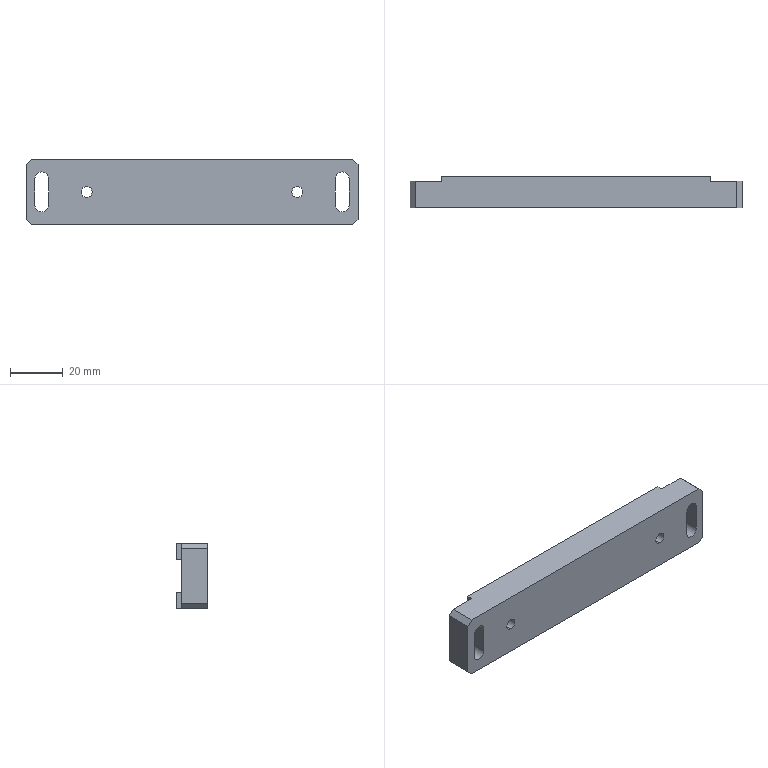Part | SolidWorks | features ICE 4, Chamfer 1, Extrusion 1, HoleWzd 1, MirrorPattern 1 | 1 solid | 32 faces | box 126 x 12 x 25 mm | volume 32289 mm3 | plane 22 | cylinder 10 | commonest cylinder face diameters 5.2 x6 4.2 x4
STEP:
#1=CARTESIAN_POINT('',(-40.,-6.,-2.1));
#2=VERTEX_POINT('',#1);
#3=CARTESIAN_POINT('',(-40.,-6.,2.1));
#4=VERTEX_POINT('',#3);
#5=CARTESIAN_POINT('',(-40.,-6.,0.));
#6=DIRECTION('',(0.,1.,0.));
#7=DIRECTION('',(0.,0.,1.));
#8=AXIS2_PLACEMENT_3D('',#5,#6,#7);
#9=CIRCLE('',#8,2.1);
#10=EDGE_CURVE('',#2,#4,#9,.T.);
#11=ORIENTED_EDGE('',*,*,#10,.F.);
#12=CARTESIAN_POINT('',(-40.,4.,-2.1));
#13=VERTEX_POINT('',#12);
#14=CARTESIAN_POINT('',(-40.,4.,-2.1));
#15=DIRECTION('',(0.,1.,0.));
#16=VECTOR('',#15,1000.);
#17=LINE('',#14,#16);
#18=EDGE_CURVE('',#2,#13,#17,.T.);
#19=ORIENTED_EDGE('',*,*,#18,.T.);
#20=CARTESIAN_POINT('',(-40.,4.,2.1));
#21=VERTEX_POINT('',#20);
#22=CARTESIAN_POINT('',(-40.,4.,0.));
#23=DIRECTION('',(0.,1.,0.));
#24=DIRECTION('',(0.,0.,1.));
#25=AXIS2_PLACEMENT_3D('',#22,#23,#24);
#26=CIRCLE('',#25,2.1);
#27=EDGE_CURVE('',#13,#21,#26,.T.);
#28=ORIENTED_EDGE('',*,*,#27,.T.);
#29=CARTESIAN_POINT('',(-40.,4.,2.1));
#30=DIRECTION('',(0.,1.,0.));
#31=VECTOR('',#30,1000.);
#32=LINE('',#29,#31);
#33=EDGE_CURVE('',#4,#21,#32,.T.);
#34=ORIENTED_EDGE('',*,*,#33,.F.);
#35=EDGE_LOOP('',(#11,#19,#28,#34));
#36=FACE_OUTER_BOUND('',#35,.T.);
#37=CARTESIAN_POINT('',(-40.,4.,0.));
#38=DIRECTION('',(0.,1.,0.));
#39=DIRECTION('',(0.,0.,1.));
#40=AXIS2_PLACEMENT_3D('',#37,#38,#39);
#41=CYLINDRICAL_SURFACE('',#40,2.1);
#42=ADVANCED_FACE('',(#36),#41,.F.);
#43=CARTESIAN_POINT('',(40.,-6.,-2.1));
#44=VERTEX_POINT('',#43);
#45=CARTESIAN_POINT('',(40.,-6.,2.1));
#46=VERTEX_POINT('',#45);
#47=CARTESIAN_POINT('',(40.,-6.,0.));
#48=DIRECTION('',(0.,1.,0.));
#49=DIRECTION('',(0.,0.,1.));
#50=AXIS2_PLACEMENT_3D('',#47,#48,#49);
#51=CIRCLE('',#50,2.1);
#52=EDGE_CURVE('',#44,#46,#51,.T.);
#53=ORIENTED_EDGE('',*,*,#52,.F.);
#54=CARTESIAN_POINT('',(40.,4.,-2.1));
#55=VERTEX_POINT('',#54);
#56=CARTESIAN_POINT('',(40.,4.,-2.1));
#57=DIRECTION('',(0.,1.,0.));
#58=VECTOR('',#57,1000.);
#59=LINE('',#56,#58);
#60=EDGE_CURVE('',#44,#55,#59,.T.);
#61=ORIENTED_EDGE('',*,*,#60,.T.);
#62=CARTESIAN_POINT('',(40.,4.,2.1));
#63=VERTEX_POINT('',#62);
#64=CARTESIAN_POINT('',(40.,4.,0.));
#65=DIRECTION('',(0.,1.,0.));
#66=DIRECTION('',(0.,0.,1.));
#67=AXIS2_PLACEMENT_3D('',#64,#65,#66);
#68=CIRCLE('',#67,2.1);
#69=EDGE_CURVE('',#55,#63,#68,.T.);
#70=ORIENTED_EDGE('',*,*,#69,.T.);
#71=CARTESIAN_POINT('',(40.,4.,2.1));
#72=DIRECTION('',(0.,1.,0.));
#73=VECTOR('',#72,1000.);
#74=LINE('',#71,#73);
#75=EDGE_CURVE('',#46,#63,#74,.T.);
#76=ORIENTED_EDGE('',*,*,#75,.F.);
#77=EDGE_LOOP('',(#53,#61,#70,#76));
#78=FACE_OUTER_BOUND('',#77,.T.);
#79=CARTESIAN_POINT('',(40.,4.,0.));
#80=DIRECTION('',(0.,1.,0.));
#81=DIRECTION('',(0.,0.,1.));
#82=AXIS2_PLACEMENT_3D('',#79,#80,#81);
#83=CYLINDRICAL_SURFACE('',#82,2.1);
#84=ADVANCED_FACE('',(#78),#83,.F.);
#85=CARTESIAN_POINT('',(59.6,-6.,5.));
#86=VERTEX_POINT('',#85);
#87=CARTESIAN_POINT('',(57.,-6.,7.6));
#88=VERTEX_POINT('',#87);
#89=CARTESIAN_POINT('',(57.,-6.,5.));
#90=DIRECTION('',(0.,-1.,0.));
#91=DIRECTION('',(0.,0.,1.));
#92=AXIS2_PLACEMENT_3D('',#89,#90,#91);
#93=CIRCLE('',#92,2.6);
#94=EDGE_CURVE('',#86,#88,#93,.T.);
#95=ORIENTED_EDGE('',*,*,#94,.T.);
#96=CARTESIAN_POINT('',(57.,4.,7.6));
#97=VERTEX_POINT('',#96);
#98=CARTESIAN_POINT('',(57.,-6.,7.6));
#99=DIRECTION('',(0.,1.,0.));
#100=VECTOR('',#99,1000.);
#101=LINE('',#98,#100);
#102=EDGE_CURVE('',#88,#97,#101,.T.);
#103=ORIENTED_EDGE('',*,*,#102,.T.);
#104=CARTESIAN_POINT('',(59.6,4.,5.));
#105=VERTEX_POINT('',#104);
#106=CARTESIAN_POINT('',(57.,4.,5.));
#107=DIRECTION('',(0.,1.,0.));
#108=DIRECTION('',(0.,0.,1.));
#109=AXIS2_PLACEMENT_3D('',#106,#107,#108);
#110=CIRCLE('',#109,2.6);
#111=EDGE_CURVE('',#97,#105,#110,.T.);
#112=ORIENTED_EDGE('',*,*,#111,.T.);
#113=CARTESIAN_POINT('',(59.6,-6.,5.));
#114=DIRECTION('',(0.,1.,0.));
#115=VECTOR('',#114,1000.);
#116=LINE('',#113,#115);
#117=EDGE_CURVE('',#86,#105,#116,.T.);
#118=ORIENTED_EDGE('',*,*,#117,.F.);
#119=EDGE_LOOP('',(#95,#103,#112,#118));
#120=FACE_OUTER_BOUND('',#119,.T.);
#121=CARTESIAN_POINT('',(57.,-6.,5.));
#122=DIRECTION('',(0.,1.,0.));
#123=DIRECTION('',(0.,0.,1.));
#124=AXIS2_PLACEMENT_3D('',#121,#122,#123);
#125=CYLINDRICAL_SURFACE('',#124,2.6);
#126=ADVANCED_FACE('',(#120),#125,.F.);
#127=CARTESIAN_POINT('',(-57.,-6.,7.6));
#128=VERTEX_POINT('',#127);
#129=CARTESIAN_POINT('',(-54.4,-6.,5.));
#130=VERTEX_POINT('',#129);
#131=CARTESIAN_POINT('',(-57.,-6.,5.));
#132=DIRECTION('',(0.,1.,0.));
#133=DIRECTION('',(0.,0.,1.));
#134=AXIS2_PLACEMENT_3D('',#131,#132,#133);
#135=CIRCLE('',#134,2.6);
#136=EDGE_CURVE('',#128,#130,#135,.T.);
#137=ORIENTED_EDGE('',*,*,#136,.F.);
#138=CARTESIAN_POINT('',(-57.,4.,7.6));
#139=VERTEX_POINT('',#138);
#140=CARTESIAN_POINT('',(-57.,-6.,7.6));
#141=DIRECTION('',(0.,1.,0.));
#142=VECTOR('',#141,1000.);
#143=LINE('',#140,#142);
#144=EDGE_CURVE('',#128,#139,#143,.T.);
#145=ORIENTED_EDGE('',*,*,#144,.T.);
#146=CARTESIAN_POINT('',(-54.4,4.,5.));
#147=VERTEX_POINT('',#146);
#148=CARTESIAN_POINT('',(-57.,4.,5.));
#149=DIRECTION('',(0.,-1.,0.));
#150=DIRECTION('',(0.,0.,1.));
#151=AXIS2_PLACEMENT_3D('',#148,#149,#150);
#152=CIRCLE('',#151,2.6);
#153=EDGE_CURVE('',#147,#139,#152,.T.);
#154=ORIENTED_EDGE('',*,*,#153,.F.);
#155=CARTESIAN_POINT('',(-54.4,-6.,5.));
#156=DIRECTION('',(0.,1.,0.));
#157=VECTOR('',#156,1000.);
#158=LINE('',#155,#157);
#159=EDGE_CURVE('',#130,#147,#158,.T.);
#160=ORIENTED_EDGE('',*,*,#159,.F.);
#161=EDGE_LOOP('',(#137,#145,#154,#160));
#162=FACE_OUTER_BOUND('',#161,.T.);
#163=CARTESIAN_POINT('',(-57.,-6.,5.));
#164=DIRECTION('',(0.,1.,0.));
#165=DIRECTION('',(0.,0.,1.));
#166=AXIS2_PLACEMENT_3D('',#163,#164,#165);
#167=CYLINDRICAL_SURFACE('',#166,2.6);
#168=ADVANCED_FACE('',(#162),#167,.F.);
#169=CARTESIAN_POINT('',(-63.,4.,-10.5));
#170=VERTEX_POINT('',#169);
#171=CARTESIAN_POINT('',(-63.,4.,10.5));
#172=VERTEX_POINT('',#171);
#173=CARTESIAN_POINT('',(-63.,4.,-12.5));
#174=DIRECTION('',(0.,0.,1.));
#175=VECTOR('',#174,1000.);
#176=LINE('',#173,#175);
#177=EDGE_CURVE('',#170,#172,#176,.T.);
#178=ORIENTED_EDGE('',*,*,#177,.F.);
#179=CARTESIAN_POINT('',(-63.,-6.,-10.5));
#180=VERTEX_POINT('',#179);
#181=CARTESIAN_POINT('',(-63.,6.,-10.5));
#182=DIRECTION('',(0.,-1.,0.));
#183=VECTOR('',#182,1000.);
#184=LINE('',#181,#183);
#185=EDGE_CURVE('',#170,#180,#184,.T.);
#186=ORIENTED_EDGE('',*,*,#185,.T.);
#187=CARTESIAN_POINT('',(-63.,-6.,10.5));
#188=VERTEX_POINT('',#187);
#189=CARTESIAN_POINT('',(-63.,-6.,-12.5));
#190=DIRECTION('',(0.,0.,1.));
#191=VECTOR('',#190,1000.);
#192=LINE('',#189,#191);
#193=EDGE_CURVE('',#180,#188,#192,.T.);
#194=ORIENTED_EDGE('',*,*,#193,.T.);
#195=CARTESIAN_POINT('',(-63.,6.,10.5));
#196=DIRECTION('',(0.,1.,0.));
#197=VECTOR('',#196,1000.);
#198=LINE('',#195,#197);
#199=EDGE_CURVE('',#188,#172,#198,.T.);
#200=ORIENTED_EDGE('',*,*,#199,.T.);
#201=EDGE_LOOP('',(#178,#186,#194,#200));
#202=FACE_OUTER_BOUND('',#201,.T.);
#203=CARTESIAN_POINT('',(-63.,6.,-12.5));
#204=DIRECTION('',(1.,0.,0.));
#205=DIRECTION('',(0.,0.,-1.));
#206=AXIS2_PLACEMENT_3D('',#203,#204,#205);
#207=PLANE('',#206);
#208=ADVANCED_FACE('',(#202),#207,.F.);
#209=CARTESIAN_POINT('',(-59.6,4.,-5.));
#210=VERTEX_POINT('',#209);
#211=CARTESIAN_POINT('',(-54.4,4.,-5.));
#212=VERTEX_POINT('',#211);
#213=CARTESIAN_POINT('',(-57.,4.,-5.));
#214=DIRECTION('',(0.,-1.,0.));
#215=DIRECTION('',(0.,0.,1.));
#216=AXIS2_PLACEMENT_3D('',#213,#214,#215);
#217=CIRCLE('',#216,2.6);
#218=EDGE_CURVE('',#210,#212,#217,.T.);
#219=ORIENTED_EDGE('',*,*,#218,.F.);
#220=CARTESIAN_POINT('',(-59.6,-6.,-5.));
#221=VERTEX_POINT('',#220);
#222=CARTESIAN_POINT('',(-59.6,-6.,-5.));
#223=DIRECTION('',(0.,1.,0.));
#224=VECTOR('',#223,1000.);
#225=LINE('',#222,#224);
#226=EDGE_CURVE('',#221,#210,#225,.T.);
#227=ORIENTED_EDGE('',*,*,#226,.F.);
#228=CARTESIAN_POINT('',(-54.4,-6.,-5.));
#229=VERTEX_POINT('',#228);
#230=CARTESIAN_POINT('',(-57.,-6.,-5.));
#231=DIRECTION('',(0.,1.,0.));
#232=DIRECTION('',(0.,0.,1.));
#233=AXIS2_PLACEMENT_3D('',#230,#231,#232);
#234=CIRCLE('',#233,2.6);
#235=EDGE_CURVE('',#229,#221,#234,.T.);
#236=ORIENTED_EDGE('',*,*,#235,.F.);
#237=CARTESIAN_POINT('',(-54.4,-6.,-5.));
#238=DIRECTION('',(0.,1.,0.));
#239=VECTOR('',#238,1000.);
#240=LINE('',#237,#239);
#241=EDGE_CURVE('',#229,#212,#240,.T.);
#242=ORIENTED_EDGE('',*,*,#241,.T.);
#243=EDGE_LOOP('',(#219,#227,#236,#242));
#244=FACE_OUTER_BOUND('',#243,.T.);
#245=CARTESIAN_POINT('',(-57.,-6.,-5.));
#246=DIRECTION('',(0.,1.,0.));
#247=DIRECTION('',(0.,0.,1.));
#248=AXIS2_PLACEMENT_3D('',#245,#246,#247);
#249=CYLINDRICAL_SURFACE('',#248,2.6);
#250=ADVANCED_FACE('',(#244),#249,.F.);
#251=ORIENTED_EDGE('',*,*,#144,.F.);
#252=CARTESIAN_POINT('',(-59.6,-6.,5.));
#253=VERTEX_POINT('',#252);
#254=CARTESIAN_POINT('',(-57.,-6.,5.));
#255=DIRECTION('',(0.,1.,0.));
#256=DIRECTION('',(0.,0.,1.));
#257=AXIS2_PLACEMENT_3D('',#254,#255,#256);
#258=CIRCLE('',#257,2.6);
#259=EDGE_CURVE('',#253,#128,#258,.T.);
#260=ORIENTED_EDGE('',*,*,#259,.F.);
#261=CARTESIAN_POINT('',(-59.6,4.,5.));
#262=VERTEX_POINT('',#261);
#263=CARTESIAN_POINT('',(-59.6,-6.,5.));
#264=DIRECTION('',(0.,1.,0.));
#265=VECTOR('',#264,1000.);
#266=LINE('',#263,#265);
#267=EDGE_CURVE('',#253,#262,#266,.T.);
#268=ORIENTED_EDGE('',*,*,#267,.T.);
#269=CARTESIAN_POINT('',(-57.,4.,5.));
#270=DIRECTION('',(0.,-1.,0.));
#271=DIRECTION('',(0.,0.,1.));
#272=AXIS2_PLACEMENT_3D('',#269,#270,#271);
#273=CIRCLE('',#272,2.6);
#274=EDGE_CURVE('',#139,#262,#273,.T.);
#275=ORIENTED_EDGE('',*,*,#274,.F.);
#276=EDGE_LOOP('',(#251,#260,#268,#275));
#277=FACE_OUTER_BOUND('',#276,.T.);
#278=CARTESIAN_POINT('',(-57.,-6.,5.));
#279=DIRECTION('',(0.,1.,0.));
#280=DIRECTION('',(0.,0.,1.));
#281=AXIS2_PLACEMENT_3D('',#278,#279,#280);
#282=CYLINDRICAL_SURFACE('',#281,2.6);
#283=ADVANCED_FACE('',(#277),#282,.F.);
#284=ORIENTED_EDGE('',*,*,#185,.F.);
#285=CARTESIAN_POINT('',(-61.,4.,-12.5));
#286=VERTEX_POINT('',#285);
#287=CARTESIAN_POINT('',(-63.,4.,-10.5));
#288=DIRECTION('',(0.7071,0.,-0.7071));
#289=VECTOR('',#288,1000.);
#290=LINE('',#287,#289);
#291=EDGE_CURVE('',#170,#286,#290,.T.);
#292=ORIENTED_EDGE('',*,*,#291,.T.);
#293=CARTESIAN_POINT('',(-61.,-6.,-12.5));
#294=VERTEX_POINT('',#293);
#295=CARTESIAN_POINT('',(-61.,6.,-12.5));
#296=DIRECTION('',(0.,1.,0.));
#297=VECTOR('',#296,1000.);
#298=LINE('',#295,#297);
#299=EDGE_CURVE('',#294,#286,#298,.T.);
#300=ORIENTED_EDGE('',*,*,#299,.F.);
#301=CARTESIAN_POINT('',(-63.,-6.,-10.5));
#302=DIRECTION('',(0.7071,0.,-0.7071));
#303=VECTOR('',#302,1000.);
#304=LINE('',#301,#303);
#305=EDGE_CURVE('',#180,#294,#304,.T.);
#306=ORIENTED_EDGE('',*,*,#305,.F.);
#307=EDGE_LOOP('',(#284,#292,#300,#306));
#308=FACE_OUTER_BOUND('',#307,.T.);
#309=CARTESIAN_POINT('',(-63.,6.,-10.5));
#310=DIRECTION('',(0.7071,0.,0.7071));
#311=DIRECTION('',(0.,-1.,0.));
#312=AXIS2_PLACEMENT_3D('',#309,#310,#311);
#313=PLANE('',#312);
#314=ADVANCED_FACE('',(#308),#313,.F.);
#315=CARTESIAN_POINT('',(-61.,4.,12.5));
#316=VERTEX_POINT('',#315);
#317=CARTESIAN_POINT('',(-61.,-6.,12.5));
#318=VERTEX_POINT('',#317);
#319=CARTESIAN_POINT('',(-61.,6.,12.5));
#320=DIRECTION('',(0.,-1.,0.));
#321=VECTOR('',#320,1000.);
#322=LINE('',#319,#321);
#323=EDGE_CURVE('',#316,#318,#322,.T.);
#324=ORIENTED_EDGE('',*,*,#323,.F.);
#325=CARTESIAN_POINT('',(-61.,4.,12.5));
#326=DIRECTION('',(-0.7071,0.,-0.7071));
#327=VECTOR('',#326,1000.);
#328=LINE('',#325,#327);
#329=EDGE_CURVE('',#316,#172,#328,.T.);
#330=ORIENTED_EDGE('',*,*,#329,.T.);
#331=ORIENTED_EDGE('',*,*,#199,.F.);
#332=CARTESIAN_POINT('',(-61.,-6.,12.5));
#333=DIRECTION('',(-0.7071,0.,-0.7071));
#334=VECTOR('',#333,1000.);
#335=LINE('',#332,#334);
#336=EDGE_CURVE('',#318,#188,#335,.T.);
#337=ORIENTED_EDGE('',*,*,#336,.F.);
#338=EDGE_LOOP('',(#324,#330,#331,#337));
#339=FACE_OUTER_BOUND('',#338,.T.);
#340=CARTESIAN_POINT('',(-61.,6.,12.5));
#341=DIRECTION('',(0.7071,0.,-0.7071));
#342=DIRECTION('',(0.,-1.,0.));
#343=AXIS2_PLACEMENT_3D('',#340,#341,#342);
#344=PLANE('',#343);
#345=ADVANCED_FACE('',(#339),#344,.F.);
#346=CARTESIAN_POINT('',(51.,6.,6.1));
#347=VERTEX_POINT('',#346);
#348=CARTESIAN_POINT('',(51.,6.,12.5));
#349=VERTEX_POINT('',#348);
#350=CARTESIAN_POINT('',(51.,6.,-53.511));
#351=DIRECTION('',(0.,0.,1.));
#352=VECTOR('',#351,1000.);
#353=LINE('',#350,#352);
#354=EDGE_CURVE('',#347,#349,#353,.T.);
#355=ORIENTED_EDGE('',*,*,#354,.F.);
#356=CARTESIAN_POINT('',(-51.,6.,6.1));
#357=VERTEX_POINT('',#356);
#358=CARTESIAN_POINT('',(-80.,6.,6.1));
#359=DIRECTION('',(1.,0.,0.));
#360=VECTOR('',#359,1000.);
#361=LINE('',#358,#360);
#362=EDGE_CURVE('',#357,#347,#361,.T.);
#363=ORIENTED_EDGE('',*,*,#362,.F.);
#364=CARTESIAN_POINT('',(-51.,6.,12.5));
#365=VERTEX_POINT('',#364);
#366=CARTESIAN_POINT('',(-51.,6.,-47.256));
#367=DIRECTION('',(0.,0.,-1.));
#368=VECTOR('',#367,1000.);
#369=LINE('',#366,#368);
#370=EDGE_CURVE('',#365,#357,#369,.T.);
#371=ORIENTED_EDGE('',*,*,#370,.F.);
#372=CARTESIAN_POINT('',(-63.,6.,12.5));
#373=DIRECTION('',(1.,0.,0.));
#374=VECTOR('',#373,1000.);
#375=LINE('',#372,#374);
#376=EDGE_CURVE('',#365,#349,#375,.T.);
#377=ORIENTED_EDGE('',*,*,#376,.T.);
#378=EDGE_LOOP('',(#355,#363,#371,#377));
#379=FACE_OUTER_BOUND('',#378,.T.);
#380=CARTESIAN_POINT('',(0.,6.,0.));
#381=DIRECTION('',(0.,1.,0.));
#382=DIRECTION('',(0.,0.,1.));
#383=AXIS2_PLACEMENT_3D('',#380,#381,#382);
#384=PLANE('',#383);
#385=ADVANCED_FACE('',(#379),#384,.T.);
#386=CARTESIAN_POINT('',(-54.4,4.,-5.));
#387=DIRECTION('',(0.,0.,1.));
#388=VECTOR('',#387,1000.);
#389=LINE('',#386,#388);
#390=EDGE_CURVE('',#212,#147,#389,.T.);
#391=ORIENTED_EDGE('',*,*,#390,.F.);
#392=ORIENTED_EDGE('',*,*,#241,.F.);
#393=CARTESIAN_POINT('',(-54.4,-6.,-5.));
#394=DIRECTION('',(0.,0.,-1.));
#395=VECTOR('',#394,1000.);
#396=LINE('',#393,#395);
#397=EDGE_CURVE('',#130,#229,#396,.T.);
#398=ORIENTED_EDGE('',*,*,#397,.F.);
#399=ORIENTED_EDGE('',*,*,#159,.T.);
#400=EDGE_LOOP('',(#391,#392,#398,#399));
#401=FACE_OUTER_BOUND('',#400,.T.);
#402=CARTESIAN_POINT('',(-54.4,-6.,-5.));
#403=DIRECTION('',(1.,0.,0.));
#404=DIRECTION('',(0.,0.,-1.));
#405=AXIS2_PLACEMENT_3D('',#402,#403,#404);
#406=PLANE('',#405);
#407=ADVANCED_FACE('',(#401),#406,.F.);
#408=CARTESIAN_POINT('',(-59.6,4.,-5.));
#409=DIRECTION('',(0.,0.,-1.));
#410=VECTOR('',#409,1000.);
#411=LINE('',#408,#410);
#412=EDGE_CURVE('',#262,#210,#411,.T.);
#413=ORIENTED_EDGE('',*,*,#412,.F.);
#414=ORIENTED_EDGE('',*,*,#267,.F.);
#415=CARTESIAN_POINT('',(-59.6,-6.,-5.));
#416=DIRECTION('',(0.,0.,1.));
#417=VECTOR('',#416,1000.);
#418=LINE('',#415,#417);
#419=EDGE_CURVE('',#221,#253,#418,.T.);
#420=ORIENTED_EDGE('',*,*,#419,.F.);
#421=ORIENTED_EDGE('',*,*,#226,.T.);
#422=EDGE_LOOP('',(#413,#414,#420,#421));
#423=FACE_OUTER_BOUND('',#422,.T.);
#424=CARTESIAN_POINT('',(-59.6,-6.,-5.));
#425=DIRECTION('',(-1.,0.,0.));
#426=DIRECTION('',(0.,0.,1.));
#427=AXIS2_PLACEMENT_3D('',#424,#425,#426);
#428=PLANE('',#427);
#429=ADVANCED_FACE('',(#423),#428,.F.);
#430=ORIENTED_EDGE('',*,*,#117,.T.);
#431=CARTESIAN_POINT('',(59.6,4.,-5.));
#432=VERTEX_POINT('',#431);
#433=CARTESIAN_POINT('',(59.6,4.,-5.));
#434=DIRECTION('',(0.,0.,-1.));
#435=VECTOR('',#434,1000.);
#436=LINE('',#433,#435);
#437=EDGE_CURVE('',#105,#432,#436,.T.);
#438=ORIENTED_EDGE('',*,*,#437,.T.);
#439=CARTESIAN_POINT('',(59.6,-6.,-5.));
#440=VERTEX_POINT('',#439);
#441=CARTESIAN_POINT('',(59.6,-6.,-5.));
#442=DIRECTION('',(0.,1.,0.));
#443=VECTOR('',#442,1000.);
#444=LINE('',#441,#443);
#445=EDGE_CURVE('',#440,#432,#444,.T.);
#446=ORIENTED_EDGE('',*,*,#445,.F.);
#447=CARTESIAN_POINT('',(59.6,-6.,-5.));
#448=DIRECTION('',(0.,0.,1.));
#449=VECTOR('',#448,1000.);
#450=LINE('',#447,#449);
#451=EDGE_CURVE('',#440,#86,#450,.T.);
#452=ORIENTED_EDGE('',*,*,#451,.T.);
#453=EDGE_LOOP('',(#430,#438,#446,#452));
#454=FACE_OUTER_BOUND('',#453,.T.);
#455=CARTESIAN_POINT('',(59.6,-6.,-5.));
#456=DIRECTION('',(-1.,0.,0.));
#457=DIRECTION('',(0.,0.,1.));
#458=AXIS2_PLACEMENT_3D('',#455,#456,#457);
#459=PLANE('',#458);
#460=ADVANCED_FACE('',(#454),#459,.T.);
#461=CARTESIAN_POINT('',(54.4,-6.,-5.));
#462=VERTEX_POINT('',#461);
#463=CARTESIAN_POINT('',(54.4,4.,-5.));
#464=VERTEX_POINT('',#463);
#465=CARTESIAN_POINT('',(54.4,-6.,-5.));
#466=DIRECTION('',(0.,1.,0.));
#467=VECTOR('',#466,1000.);
#468=LINE('',#465,#467);
#469=EDGE_CURVE('',#462,#464,#468,.T.);
#470=ORIENTED_EDGE('',*,*,#469,.T.);
#471=CARTESIAN_POINT('',(54.4,4.,5.));
#472=VERTEX_POINT('',#471);
#473=CARTESIAN_POINT('',(54.4,4.,-5.));
#474=DIRECTION('',(0.,0.,1.));
#475=VECTOR('',#474,1000.);
#476=LINE('',#473,#475);
#477=EDGE_CURVE('',#464,#472,#476,.T.);
#478=ORIENTED_EDGE('',*,*,#477,.T.);
#479=CARTESIAN_POINT('',(54.4,-6.,5.));
#480=VERTEX_POINT('',#479);
#481=CARTESIAN_POINT('',(54.4,-6.,5.));
#482=DIRECTION('',(0.,1.,0.));
#483=VECTOR('',#482,1000.);
#484=LINE('',#481,#483);
#485=EDGE_CURVE('',#480,#472,#484,.T.);
#486=ORIENTED_EDGE('',*,*,#485,.F.);
#487=CARTESIAN_POINT('',(54.4,-6.,-5.));
#488=DIRECTION('',(0.,0.,-1.));
#489=VECTOR('',#488,1000.);
#490=LINE('',#487,#489);
#491=EDGE_CURVE('',#480,#462,#490,.T.);
#492=ORIENTED_EDGE('',*,*,#491,.T.);
#493=EDGE_LOOP('',(#470,#478,#486,#492));
#494=FACE_OUTER_BOUND('',#493,.T.);
#495=CARTESIAN_POINT('',(54.4,-6.,-5.));
#496=DIRECTION('',(1.,0.,0.));
#497=DIRECTION('',(0.,0.,-1.));
#498=AXIS2_PLACEMENT_3D('',#495,#496,#497);
#499=PLANE('',#498);
#500=ADVANCED_FACE('',(#494),#499,.T.);
#501=CARTESIAN_POINT('',(51.,6.,-12.5));
#502=VERTEX_POINT('',#501);
#503=CARTESIAN_POINT('',(51.,6.,-6.1));
#504=VERTEX_POINT('',#503);
#505=CARTESIAN_POINT('',(51.,6.,-53.511));
#506=DIRECTION('',(0.,0.,1.));
#507=VECTOR('',#506,1000.);
#508=LINE('',#505,#507);
#509=EDGE_CURVE('',#502,#504,#508,.T.);
#510=ORIENTED_EDGE('',*,*,#509,.F.);
#511=CARTESIAN_POINT('',(-51.,6.,-12.5));
#512=VERTEX_POINT('',#511);
#513=CARTESIAN_POINT('',(-63.,6.,-12.5));
#514=DIRECTION('',(-1.,0.,0.));
#515=VECTOR('',#514,1000.);
#516=LINE('',#513,#515);
#517=EDGE_CURVE('',#502,#512,#516,.T.);
#518=ORIENTED_EDGE('',*,*,#517,.T.);
#519=CARTESIAN_POINT('',(-51.,6.,-6.1));
#520=VERTEX_POINT('',#519);
#521=CARTESIAN_POINT('',(-51.,6.,-47.256));
#522=DIRECTION('',(0.,0.,-1.));
#523=VECTOR('',#522,1000.);
#524=LINE('',#521,#523);
#525=EDGE_CURVE('',#520,#512,#524,.T.);
#526=ORIENTED_EDGE('',*,*,#525,.F.);
#527=CARTESIAN_POINT('',(-80.,6.,-6.1));
#528=DIRECTION('',(-1.,0.,0.));
#529=VECTOR('',#528,1000.);
#530=LINE('',#527,#529);
#531=EDGE_CURVE('',#504,#520,#530,.T.);
#532=ORIENTED_EDGE('',*,*,#531,.F.);
#533=EDGE_LOOP('',(#510,#518,#526,#532));
#534=FACE_OUTER_BOUND('',#533,.T.);
#535=CARTESIAN_POINT('',(0.,6.,0.));
#536=DIRECTION('',(0.,1.,0.));
#537=DIRECTION('',(0.,0.,1.));
#538=AXIS2_PLACEMENT_3D('',#535,#536,#537);
#539=PLANE('',#538);
#540=ADVANCED_FACE('',(#534),#539,.T.);
#541=CARTESIAN_POINT('',(-40.,-6.,0.));
#542=DIRECTION('',(0.,1.,0.));
#543=DIRECTION('',(0.,0.,1.));
#544=AXIS2_PLACEMENT_3D('',#541,#542,#543);
#545=CIRCLE('',#544,2.1);
#546=EDGE_CURVE('',#4,#2,#545,.T.);
#547=ORIENTED_EDGE('',*,*,#546,.T.);
#548=ORIENTED_EDGE('',*,*,#10,.T.);
#549=EDGE_LOOP('',(#547,#548));
#550=FACE_BOUND('',#549,.T.);
#551=CARTESIAN_POINT('',(40.,-6.,0.));
#552=DIRECTION('',(0.,1.,0.));
#553=DIRECTION('',(0.,0.,1.));
#554=AXIS2_PLACEMENT_3D('',#551,#552,#553);
#555=CIRCLE('',#554,2.1);
#556=EDGE_CURVE('',#46,#44,#555,.T.);
#557=ORIENTED_EDGE('',*,*,#556,.T.);
#558=ORIENTED_EDGE('',*,*,#52,.T.);
#559=EDGE_LOOP('',(#557,#558));
#560=FACE_BOUND('',#559,.T.);
#561=ORIENTED_EDGE('',*,*,#193,.F.);
#562=ORIENTED_EDGE('',*,*,#305,.T.);
#563=CARTESIAN_POINT('',(61.,-6.,-12.5));
#564=VERTEX_POINT('',#563);
#565=CARTESIAN_POINT('',(-63.,-6.,-12.5));
#566=DIRECTION('',(-1.,0.,0.));
#567=VECTOR('',#566,1000.);
#568=LINE('',#565,#567);
#569=EDGE_CURVE('',#564,#294,#568,.T.);
#570=ORIENTED_EDGE('',*,*,#569,.F.);
#571=CARTESIAN_POINT('',(63.,-6.,-10.5));
#572=VERTEX_POINT('',#571);
#573=CARTESIAN_POINT('',(61.,-6.,-12.5));
#574=DIRECTION('',(0.7071,0.,0.7071));
#575=VECTOR('',#574,1000.);
#576=LINE('',#573,#575);
#577=EDGE_CURVE('',#564,#572,#576,.T.);
#578=ORIENTED_EDGE('',*,*,#577,.T.);
#579=CARTESIAN_POINT('',(63.,-6.,10.5));
#580=VERTEX_POINT('',#579);
#581=CARTESIAN_POINT('',(63.,-6.,-12.5));
#582=DIRECTION('',(0.,0.,-1.));
#583=VECTOR('',#582,1000.);
#584=LINE('',#581,#583);
#585=EDGE_CURVE('',#580,#572,#584,.T.);
#586=ORIENTED_EDGE('',*,*,#585,.F.);
#587=CARTESIAN_POINT('',(61.,-6.,12.5));
#588=VERTEX_POINT('',#587);
#589=CARTESIAN_POINT('',(63.,-6.,10.5));
#590=DIRECTION('',(-0.7071,0.,0.7071));
#591=VECTOR('',#590,1000.);
#592=LINE('',#589,#591);
#593=EDGE_CURVE('',#580,#588,#592,.T.);
#594=ORIENTED_EDGE('',*,*,#593,.T.);
#595=CARTESIAN_POINT('',(-63.,-6.,12.5));
#596=DIRECTION('',(1.,0.,0.));
#597=VECTOR('',#596,1000.);
#598=LINE('',#595,#597);
#599=EDGE_CURVE('',#318,#588,#598,.T.);
#600=ORIENTED_EDGE('',*,*,#599,.F.);
#601=ORIENTED_EDGE('',*,*,#336,.T.);
#602=EDGE_LOOP('',(#561,#562,#570,#578,#586,#594,#600,#601));
#603=FACE_OUTER_BOUND('',#602,.T.);
#604=ORIENTED_EDGE('',*,*,#397,.T.);
#605=ORIENTED_EDGE('',*,*,#235,.T.);
#606=ORIENTED_EDGE('',*,*,#419,.T.);
#607=ORIENTED_EDGE('',*,*,#259,.T.);
#608=ORIENTED_EDGE('',*,*,#136,.T.);
#609=EDGE_LOOP('',(#604,#605,#606,#607,#608));
#610=FACE_BOUND('',#609,.T.);
#611=CARTESIAN_POINT('',(57.,-6.,-5.));
#612=DIRECTION('',(0.,-1.,0.));
#613=DIRECTION('',(0.,0.,1.));
#614=AXIS2_PLACEMENT_3D('',#611,#612,#613);
#615=CIRCLE('',#614,2.6);
#616=EDGE_CURVE('',#462,#440,#615,.T.);
#617=ORIENTED_EDGE('',*,*,#616,.F.);
#618=ORIENTED_EDGE('',*,*,#491,.F.);
#619=CARTESIAN_POINT('',(57.,-6.,5.));
#620=DIRECTION('',(0.,-1.,0.));
#621=DIRECTION('',(0.,0.,1.));
#622=AXIS2_PLACEMENT_3D('',#619,#620,#621);
#623=CIRCLE('',#622,2.6);
#624=EDGE_CURVE('',#88,#480,#623,.T.);
#625=ORIENTED_EDGE('',*,*,#624,.F.);
#626=ORIENTED_EDGE('',*,*,#94,.F.);
#627=ORIENTED_EDGE('',*,*,#451,.F.);
#628=EDGE_LOOP('',(#617,#618,#625,#626,#627));
#629=FACE_BOUND('',#628,.T.);
#630=CARTESIAN_POINT('',(0.,-6.,0.));
#631=DIRECTION('',(0.,1.,0.));
#632=DIRECTION('',(0.,0.,1.));
#633=AXIS2_PLACEMENT_3D('',#630,#631,#632);
#634=PLANE('',#633);
#635=ADVANCED_FACE('',(#550,#560,#603,#610,#629),#634,.F.);
#636=CARTESIAN_POINT('',(63.,4.,-10.5));
#637=VERTEX_POINT('',#636);
#638=CARTESIAN_POINT('',(63.,6.,-10.5));
#639=DIRECTION('',(0.,1.,0.));
#640=VECTOR('',#639,1000.);
#641=LINE('',#638,#640);
#642=EDGE_CURVE('',#572,#637,#641,.T.);
#643=ORIENTED_EDGE('',*,*,#642,.T.);
#644=CARTESIAN_POINT('',(63.,4.,10.5));
#645=VERTEX_POINT('',#644);
#646=CARTESIAN_POINT('',(63.,4.,-12.5));
#647=DIRECTION('',(0.,0.,-1.));
#648=VECTOR('',#647,1000.);
#649=LINE('',#646,#648);
#650=EDGE_CURVE('',#645,#637,#649,.T.);
#651=ORIENTED_EDGE('',*,*,#650,.F.);
#652=CARTESIAN_POINT('',(63.,6.,10.5));
#653=DIRECTION('',(0.,-1.,0.));
#654=VECTOR('',#653,1000.);
#655=LINE('',#652,#654);
#656=EDGE_CURVE('',#645,#580,#655,.T.);
#657=ORIENTED_EDGE('',*,*,#656,.T.);
#658=ORIENTED_EDGE('',*,*,#585,.T.);
#659=EDGE_LOOP('',(#643,#651,#657,#658));
#660=FACE_OUTER_BOUND('',#659,.T.);
#661=CARTESIAN_POINT('',(63.,6.,-12.5));
#662=DIRECTION('',(-1.,0.,0.));
#663=DIRECTION('',(0.,0.,1.));
#664=AXIS2_PLACEMENT_3D('',#661,#662,#663);
#665=PLANE('',#664);
#666=ADVANCED_FACE('',(#660),#665,.F.);
#667=ORIENTED_EDGE('',*,*,#517,.F.);
#668=CARTESIAN_POINT('',(51.,4.,-12.5));
#669=VERTEX_POINT('',#668);
#670=CARTESIAN_POINT('',(51.,6.,-12.5));
#671=DIRECTION('',(0.,-1.,0.));
#672=VECTOR('',#671,1000.);
#673=LINE('',#670,#672);
#674=EDGE_CURVE('',#502,#669,#673,.T.);
#675=ORIENTED_EDGE('',*,*,#674,.T.);
#676=CARTESIAN_POINT('',(61.,4.,-12.5));
#677=VERTEX_POINT('',#676);
#678=CARTESIAN_POINT('',(-63.,4.,-12.5));
#679=DIRECTION('',(1.,0.,0.));
#680=VECTOR('',#679,1000.);
#681=LINE('',#678,#680);
#682=EDGE_CURVE('',#669,#677,#681,.T.);
#683=ORIENTED_EDGE('',*,*,#682,.T.);
#684=CARTESIAN_POINT('',(61.,6.,-12.5));
#685=DIRECTION('',(0.,-1.,0.));
#686=VECTOR('',#685,1000.);
#687=LINE('',#684,#686);
#688=EDGE_CURVE('',#677,#564,#687,.T.);
#689=ORIENTED_EDGE('',*,*,#688,.T.);
#690=ORIENTED_EDGE('',*,*,#569,.T.);
#691=ORIENTED_EDGE('',*,*,#299,.T.);
#692=CARTESIAN_POINT('',(-51.,4.,-12.5));
#693=VERTEX_POINT('',#692);
#694=CARTESIAN_POINT('',(-63.,4.,-12.5));
#695=DIRECTION('',(-1.,0.,0.));
#696=VECTOR('',#695,1000.);
#697=LINE('',#694,#696);
#698=EDGE_CURVE('',#693,#286,#697,.T.);
#699=ORIENTED_EDGE('',*,*,#698,.F.);
#700=CARTESIAN_POINT('',(-51.,6.,-12.5));
#701=DIRECTION('',(0.,1.,0.));
#702=VECTOR('',#701,1000.);
#703=LINE('',#700,#702);
#704=EDGE_CURVE('',#693,#512,#703,.T.);
#705=ORIENTED_EDGE('',*,*,#704,.T.);
#706=EDGE_LOOP('',(#667,#675,#683,#689,#690,#691,#699,#705));
#707=FACE_OUTER_BOUND('',#706,.T.);
#708=CARTESIAN_POINT('',(-63.,6.,-12.5));
#709=DIRECTION('',(0.,0.,1.));
#710=DIRECTION('',(1.,0.,0.));
#711=AXIS2_PLACEMENT_3D('',#708,#709,#710);
#712=PLANE('',#711);
#713=ADVANCED_FACE('',(#707),#712,.F.);
#714=CARTESIAN_POINT('',(61.,4.,12.5));
#715=VERTEX_POINT('',#714);
#716=CARTESIAN_POINT('',(51.,4.,12.5));
#717=VERTEX_POINT('',#716);
#718=CARTESIAN_POINT('',(-63.,4.,12.5));
#719=DIRECTION('',(-1.,0.,0.));
#720=VECTOR('',#719,1000.);
#721=LINE('',#718,#720);
#722=EDGE_CURVE('',#715,#717,#721,.T.);
#723=ORIENTED_EDGE('',*,*,#722,.T.);
#724=CARTESIAN_POINT('',(51.,6.,12.5));
#725=DIRECTION('',(0.,1.,0.));
#726=VECTOR('',#725,1000.);
#727=LINE('',#724,#726);
#728=EDGE_CURVE('',#717,#349,#727,.T.);
#729=ORIENTED_EDGE('',*,*,#728,.T.);
#730=ORIENTED_EDGE('',*,*,#376,.F.);
#731=CARTESIAN_POINT('',(-51.,4.,12.5));
#732=VERTEX_POINT('',#731);
#733=CARTESIAN_POINT('',(-51.,6.,12.5));
#734=DIRECTION('',(0.,-1.,0.));
#735=VECTOR('',#734,1000.);
#736=LINE('',#733,#735);
#737=EDGE_CURVE('',#365,#732,#736,.T.);
#738=ORIENTED_EDGE('',*,*,#737,.T.);
#739=CARTESIAN_POINT('',(-63.,4.,12.5));
#740=DIRECTION('',(1.,0.,0.));
#741=VECTOR('',#740,1000.);
#742=LINE('',#739,#741);
#743=EDGE_CURVE('',#316,#732,#742,.T.);
#744=ORIENTED_EDGE('',*,*,#743,.F.);
#745=ORIENTED_EDGE('',*,*,#323,.T.);
#746=ORIENTED_EDGE('',*,*,#599,.T.);
#747=CARTESIAN_POINT('',(61.,6.,12.5));
#748=DIRECTION('',(0.,1.,0.));
#749=VECTOR('',#748,1000.);
#750=LINE('',#747,#749);
#751=EDGE_CURVE('',#588,#715,#750,.T.);
#752=ORIENTED_EDGE('',*,*,#751,.T.);
#753=EDGE_LOOP('',(#723,#729,#730,#738,#744,#745,#746,#752));
#754=FACE_OUTER_BOUND('',#753,.T.);
#755=CARTESIAN_POINT('',(-63.,6.,12.5));
#756=DIRECTION('',(0.,0.,-1.));
#757=DIRECTION('',(-1.,0.,0.));
#758=AXIS2_PLACEMENT_3D('',#755,#756,#757);
#759=PLANE('',#758);
#760=ADVANCED_FACE('',(#754),#759,.F.);
#761=CARTESIAN_POINT('',(57.,4.,-5.));
#762=DIRECTION('',(0.,1.,0.));
#763=DIRECTION('',(0.,0.,1.));
#764=AXIS2_PLACEMENT_3D('',#761,#762,#763);
#765=CIRCLE('',#764,2.6);
#766=EDGE_CURVE('',#432,#464,#765,.T.);
#767=ORIENTED_EDGE('',*,*,#766,.T.);
#768=ORIENTED_EDGE('',*,*,#469,.F.);
#769=ORIENTED_EDGE('',*,*,#616,.T.);
#770=ORIENTED_EDGE('',*,*,#445,.T.);
#771=EDGE_LOOP('',(#767,#768,#769,#770));
#772=FACE_OUTER_BOUND('',#771,.T.);
#773=CARTESIAN_POINT('',(57.,-6.,-5.));
#774=DIRECTION('',(0.,1.,0.));
#775=DIRECTION('',(0.,0.,1.));
#776=AXIS2_PLACEMENT_3D('',#773,#774,#775);
#777=CYLINDRICAL_SURFACE('',#776,2.6);
#778=ADVANCED_FACE('',(#772),#777,.F.);
#779=ORIENTED_EDGE('',*,*,#102,.F.);
#780=ORIENTED_EDGE('',*,*,#624,.T.);
#781=ORIENTED_EDGE('',*,*,#485,.T.);
#782=CARTESIAN_POINT('',(57.,4.,5.));
#783=DIRECTION('',(0.,1.,0.));
#784=DIRECTION('',(0.,0.,1.));
#785=AXIS2_PLACEMENT_3D('',#782,#783,#784);
#786=CIRCLE('',#785,2.6);
#787=EDGE_CURVE('',#472,#97,#786,.T.);
#788=ORIENTED_EDGE('',*,*,#787,.T.);
#789=EDGE_LOOP('',(#779,#780,#781,#788));
#790=FACE_OUTER_BOUND('',#789,.T.);
#791=CARTESIAN_POINT('',(57.,-6.,5.));
#792=DIRECTION('',(0.,1.,0.));
#793=DIRECTION('',(0.,0.,1.));
#794=AXIS2_PLACEMENT_3D('',#791,#792,#793);
#795=CYLINDRICAL_SURFACE('',#794,2.6);
#796=ADVANCED_FACE('',(#790),#795,.F.);
#797=ORIENTED_EDGE('',*,*,#362,.T.);
#798=CARTESIAN_POINT('',(51.,4.,6.1));
#799=VERTEX_POINT('',#798);
#800=CARTESIAN_POINT('',(51.,4.,6.1));
#801=DIRECTION('',(0.,-1.,0.));
#802=VECTOR('',#801,1000.);
#803=LINE('',#800,#802);
#804=EDGE_CURVE('',#347,#799,#803,.T.);
#805=ORIENTED_EDGE('',*,*,#804,.T.);
#806=CARTESIAN_POINT('',(-51.,4.,6.1));
#807=VERTEX_POINT('',#806);
#808=CARTESIAN_POINT('',(-80.,4.,6.1));
#809=DIRECTION('',(1.,0.,0.));
#810=VECTOR('',#809,1000.);
#811=LINE('',#808,#810);
#812=EDGE_CURVE('',#807,#799,#811,.T.);
#813=ORIENTED_EDGE('',*,*,#812,.F.);
#814=CARTESIAN_POINT('',(-51.,4.,6.1));
#815=DIRECTION('',(0.,1.,0.));
#816=VECTOR('',#815,1000.);
#817=LINE('',#814,#816);
#818=EDGE_CURVE('',#807,#357,#817,.T.);
#819=ORIENTED_EDGE('',*,*,#818,.T.);
#820=EDGE_LOOP('',(#797,#805,#813,#819));
#821=FACE_OUTER_BOUND('',#820,.T.);
#822=CARTESIAN_POINT('',(-80.,4.,6.1));
#823=DIRECTION('',(0.,0.,1.));
#824=DIRECTION('',(1.,0.,0.));
#825=AXIS2_PLACEMENT_3D('',#822,#823,#824);
#826=PLANE('',#825);
#827=ADVANCED_FACE('',(#821),#826,.F.);
#828=CARTESIAN_POINT('',(51.,4.,-6.1));
#829=VERTEX_POINT('',#828);
#830=CARTESIAN_POINT('',(-51.,4.,-6.1));
#831=VERTEX_POINT('',#830);
#832=CARTESIAN_POINT('',(-80.,4.,-6.1));
#833=DIRECTION('',(-1.,0.,0.));
#834=VECTOR('',#833,1000.);
#835=LINE('',#832,#834);
#836=EDGE_CURVE('',#829,#831,#835,.T.);
#837=ORIENTED_EDGE('',*,*,#836,.F.);
#838=CARTESIAN_POINT('',(51.,4.,-6.1));
#839=DIRECTION('',(0.,1.,0.));
#840=VECTOR('',#839,1000.);
#841=LINE('',#838,#840);
#842=EDGE_CURVE('',#829,#504,#841,.T.);
#843=ORIENTED_EDGE('',*,*,#842,.T.);
#844=ORIENTED_EDGE('',*,*,#531,.T.);
#845=CARTESIAN_POINT('',(-51.,4.,-6.1));
#846=DIRECTION('',(0.,-1.,0.));
#847=VECTOR('',#846,1000.);
#848=LINE('',#845,#847);
#849=EDGE_CURVE('',#520,#831,#848,.T.);
#850=ORIENTED_EDGE('',*,*,#849,.T.);
#851=EDGE_LOOP('',(#837,#843,#844,#850));
#852=FACE_OUTER_BOUND('',#851,.T.);
#853=CARTESIAN_POINT('',(-80.,4.,-6.1));
#854=DIRECTION('',(0.,0.,-1.));
#855=DIRECTION('',(-1.,0.,0.));
#856=AXIS2_PLACEMENT_3D('',#853,#854,#855);
#857=PLANE('',#856);
#858=ADVANCED_FACE('',(#852),#857,.F.);
#859=ORIENTED_EDGE('',*,*,#787,.F.);
#860=ORIENTED_EDGE('',*,*,#477,.F.);
#861=ORIENTED_EDGE('',*,*,#766,.F.);
#862=ORIENTED_EDGE('',*,*,#437,.F.);
#863=ORIENTED_EDGE('',*,*,#111,.F.);
#864=EDGE_LOOP('',(#859,#860,#861,#862,#863));
#865=FACE_BOUND('',#864,.T.);
#866=ORIENTED_EDGE('',*,*,#650,.T.);
#867=CARTESIAN_POINT('',(61.,4.,-12.5));
#868=DIRECTION('',(-0.7071,0.,-0.7071));
#869=VECTOR('',#868,1000.);
#870=LINE('',#867,#869);
#871=EDGE_CURVE('',#637,#677,#870,.T.);
#872=ORIENTED_EDGE('',*,*,#871,.T.);
#873=ORIENTED_EDGE('',*,*,#682,.F.);
#874=CARTESIAN_POINT('',(51.,4.,-53.511));
#875=DIRECTION('',(0.,0.,1.));
#876=VECTOR('',#875,1000.);
#877=LINE('',#874,#876);
#878=EDGE_CURVE('',#669,#829,#877,.T.);
#879=ORIENTED_EDGE('',*,*,#878,.T.);
#880=ORIENTED_EDGE('',*,*,#836,.T.);
#881=CARTESIAN_POINT('',(-51.,4.,-47.256));
#882=DIRECTION('',(0.,0.,-1.));
#883=VECTOR('',#882,1000.);
#884=LINE('',#881,#883);
#885=EDGE_CURVE('',#831,#693,#884,.T.);
#886=ORIENTED_EDGE('',*,*,#885,.T.);
#887=ORIENTED_EDGE('',*,*,#698,.T.);
#888=ORIENTED_EDGE('',*,*,#291,.F.);
#889=ORIENTED_EDGE('',*,*,#177,.T.);
#890=ORIENTED_EDGE('',*,*,#329,.F.);
#891=ORIENTED_EDGE('',*,*,#743,.T.);
#892=CARTESIAN_POINT('',(-51.,4.,-47.256));
#893=DIRECTION('',(0.,0.,-1.));
#894=VECTOR('',#893,1000.);
#895=LINE('',#892,#894);
#896=EDGE_CURVE('',#732,#807,#895,.T.);
#897=ORIENTED_EDGE('',*,*,#896,.T.);
#898=ORIENTED_EDGE('',*,*,#812,.T.);
#899=CARTESIAN_POINT('',(51.,4.,-53.511));
#900=DIRECTION('',(0.,0.,1.));
#901=VECTOR('',#900,1000.);
#902=LINE('',#899,#901);
#903=EDGE_CURVE('',#799,#717,#902,.T.);
#904=ORIENTED_EDGE('',*,*,#903,.T.);
#905=ORIENTED_EDGE('',*,*,#722,.F.);
#906=CARTESIAN_POINT('',(63.,4.,10.5));
#907=DIRECTION('',(0.7071,0.,-0.7071));
#908=VECTOR('',#907,1000.);
#909=LINE('',#906,#908);
#910=EDGE_CURVE('',#715,#645,#909,.T.);
#911=ORIENTED_EDGE('',*,*,#910,.T.);
#912=EDGE_LOOP('',(#866,#872,#873,#879,#880,#886,#887,#888,#889,#890,#891,#897,#898,#904,#905,#911));
#913=FACE_OUTER_BOUND('',#912,.T.);
#914=ORIENTED_EDGE('',*,*,#153,.T.);
#915=ORIENTED_EDGE('',*,*,#274,.T.);
#916=ORIENTED_EDGE('',*,*,#412,.T.);
#917=ORIENTED_EDGE('',*,*,#218,.T.);
#918=ORIENTED_EDGE('',*,*,#390,.T.);
#919=EDGE_LOOP('',(#914,#915,#916,#917,#918));
#920=FACE_BOUND('',#919,.T.);
#921=CARTESIAN_POINT('',(-40.,4.,0.));
#922=DIRECTION('',(0.,1.,0.));
#923=DIRECTION('',(0.,0.,1.));
#924=AXIS2_PLACEMENT_3D('',#921,#922,#923);
#925=CIRCLE('',#924,2.1);
#926=EDGE_CURVE('',#21,#13,#925,.T.);
#927=ORIENTED_EDGE('',*,*,#926,.F.);
#928=ORIENTED_EDGE('',*,*,#27,.F.);
#929=EDGE_LOOP('',(#927,#928));
#930=FACE_BOUND('',#929,.T.);
#931=CARTESIAN_POINT('',(40.,4.,0.));
#932=DIRECTION('',(0.,1.,0.));
#933=DIRECTION('',(0.,0.,1.));
#934=AXIS2_PLACEMENT_3D('',#931,#932,#933);
#935=CIRCLE('',#934,2.1);
#936=EDGE_CURVE('',#63,#55,#935,.T.);
#937=ORIENTED_EDGE('',*,*,#936,.F.);
#938=ORIENTED_EDGE('',*,*,#69,.F.);
#939=EDGE_LOOP('',(#937,#938));
#940=FACE_BOUND('',#939,.T.);
#941=CARTESIAN_POINT('',(0.,4.,0.));
#942=DIRECTION('',(0.,1.,0.));
#943=DIRECTION('',(0.,0.,1.));
#944=AXIS2_PLACEMENT_3D('',#941,#942,#943);
#945=PLANE('',#944);
#946=ADVANCED_FACE('',(#865,#913,#920,#930,#940),#945,.T.);
#947=ORIENTED_EDGE('',*,*,#871,.F.);
#948=ORIENTED_EDGE('',*,*,#642,.F.);
#949=ORIENTED_EDGE('',*,*,#577,.F.);
#950=ORIENTED_EDGE('',*,*,#688,.F.);
#951=EDGE_LOOP('',(#947,#948,#949,#950));
#952=FACE_OUTER_BOUND('',#951,.T.);
#953=CARTESIAN_POINT('',(61.,6.,-12.5));
#954=DIRECTION('',(-0.7071,0.,0.7071));
#955=DIRECTION('',(0.,-1.,0.));
#956=AXIS2_PLACEMENT_3D('',#953,#954,#955);
#957=PLANE('',#956);
#958=ADVANCED_FACE('',(#952),#957,.F.);
#959=ORIENTED_EDGE('',*,*,#910,.F.);
#960=ORIENTED_EDGE('',*,*,#751,.F.);
#961=ORIENTED_EDGE('',*,*,#593,.F.);
#962=ORIENTED_EDGE('',*,*,#656,.F.);
#963=EDGE_LOOP('',(#959,#960,#961,#962));
#964=FACE_OUTER_BOUND('',#963,.T.);
#965=CARTESIAN_POINT('',(63.,6.,10.5));
#966=DIRECTION('',(-0.7071,0.,-0.7071));
#967=DIRECTION('',(0.,-1.,0.));
#968=AXIS2_PLACEMENT_3D('',#965,#966,#967);
#969=PLANE('',#968);
#970=ADVANCED_FACE('',(#964),#969,.F.);
#971=ORIENTED_EDGE('',*,*,#60,.F.);
#972=ORIENTED_EDGE('',*,*,#556,.F.);
#973=ORIENTED_EDGE('',*,*,#75,.T.);
#974=ORIENTED_EDGE('',*,*,#936,.T.);
#975=EDGE_LOOP('',(#971,#972,#973,#974));
#976=FACE_OUTER_BOUND('',#975,.T.);
#977=CARTESIAN_POINT('',(40.,4.,0.));
#978=DIRECTION('',(0.,1.,0.));
#979=DIRECTION('',(0.,0.,1.));
#980=AXIS2_PLACEMENT_3D('',#977,#978,#979);
#981=CYLINDRICAL_SURFACE('',#980,2.1);
#982=ADVANCED_FACE('',(#976),#981,.F.);
#983=ORIENTED_EDGE('',*,*,#18,.F.);
#984=ORIENTED_EDGE('',*,*,#546,.F.);
#985=ORIENTED_EDGE('',*,*,#33,.T.);
#986=ORIENTED_EDGE('',*,*,#926,.T.);
#987=EDGE_LOOP('',(#983,#984,#985,#986));
#988=FACE_OUTER_BOUND('',#987,.T.);
#989=CARTESIAN_POINT('',(-40.,4.,0.));
#990=DIRECTION('',(0.,1.,0.));
#991=DIRECTION('',(0.,0.,1.));
#992=AXIS2_PLACEMENT_3D('',#989,#990,#991);
#993=CYLINDRICAL_SURFACE('',#992,2.1);
#994=ADVANCED_FACE('',(#988),#993,.F.);
#995=ORIENTED_EDGE('',*,*,#370,.T.);
#996=ORIENTED_EDGE('',*,*,#818,.F.);
#997=ORIENTED_EDGE('',*,*,#896,.F.);
#998=ORIENTED_EDGE('',*,*,#737,.F.);
#999=EDGE_LOOP('',(#995,#996,#997,#998));
#1000=FACE_OUTER_BOUND('',#999,.T.);
#1001=CARTESIAN_POINT('',(-51.,4.,-47.256));
#1002=DIRECTION('',(1.,0.,0.));
#1003=DIRECTION('',(0.,0.,-1.));
#1004=AXIS2_PLACEMENT_3D('',#1001,#1002,#1003);
#1005=PLANE('',#1004);
#1006=ADVANCED_FACE('',(#1000),#1005,.F.);
#1007=ORIENTED_EDGE('',*,*,#885,.F.);
#1008=ORIENTED_EDGE('',*,*,#849,.F.);
#1009=ORIENTED_EDGE('',*,*,#525,.T.);
#1010=ORIENTED_EDGE('',*,*,#704,.F.);
#1011=EDGE_LOOP('',(#1007,#1008,#1009,#1010));
#1012=FACE_OUTER_BOUND('',#1011,.T.);
#1013=CARTESIAN_POINT('',(-51.,4.,-47.256));
#1014=DIRECTION('',(1.,0.,0.));
#1015=DIRECTION('',(0.,0.,-1.));
#1016=AXIS2_PLACEMENT_3D('',#1013,#1014,#1015);
#1017=PLANE('',#1016);
#1018=ADVANCED_FACE('',(#1012),#1017,.F.);
#1019=ORIENTED_EDGE('',*,*,#903,.F.);
#1020=ORIENTED_EDGE('',*,*,#804,.F.);
#1021=ORIENTED_EDGE('',*,*,#354,.T.);
#1022=ORIENTED_EDGE('',*,*,#728,.F.);
#1023=EDGE_LOOP('',(#1019,#1020,#1021,#1022));
#1024=FACE_OUTER_BOUND('',#1023,.T.);
#1025=CARTESIAN_POINT('',(51.,4.,-53.511));
#1026=DIRECTION('',(-1.,0.,0.));
#1027=DIRECTION('',(0.,0.,1.));
#1028=AXIS2_PLACEMENT_3D('',#1025,#1026,#1027);
#1029=PLANE('',#1028);
#1030=ADVANCED_FACE('',(#1024),#1029,.F.);
#1031=ORIENTED_EDGE('',*,*,#509,.T.);
#1032=ORIENTED_EDGE('',*,*,#842,.F.);
#1033=ORIENTED_EDGE('',*,*,#878,.F.);
#1034=ORIENTED_EDGE('',*,*,#674,.F.);
#1035=EDGE_LOOP('',(#1031,#1032,#1033,#1034));
#1036=FACE_OUTER_BOUND('',#1035,.T.);
#1037=CARTESIAN_POINT('',(51.,4.,-53.511));
#1038=DIRECTION('',(-1.,0.,0.));
#1039=DIRECTION('',(0.,0.,1.));
#1040=AXIS2_PLACEMENT_3D('',#1037,#1038,#1039);
#1041=PLANE('',#1040);
#1042=ADVANCED_FACE('',(#1036),#1041,.F.);
#1043=CLOSED_SHELL('',(#42,#84,#126,#168,#208,#250,#283,#314,#345,#385,#407,#429,#460,#500,#540,#635,#666,#713,#760,#778,#796,#827,#858,#946,#958,#970,#982,#994,#1006,#1018,#1030,#1042));
#1044=MANIFOLD_SOLID_BREP('',#1043);
#1045=CARTESIAN_POINT('',(0.,0.,0.));
#1046=DIRECTION('',(0.,0.,1.));
#1047=DIRECTION('',(1.,0.,0.));
#1048=AXIS2_PLACEMENT_3D('',#1045,#1046,#1047);
#1049=(LENGTH_UNIT()NAMED_UNIT(*)SI_UNIT(.MILLI.,.METRE.));
#1050=UNCERTAINTY_MEASURE_WITH_UNIT(LENGTH_MEASURE(0.00001),#1049,'','');
#1051=(NAMED_UNIT(*)PLANE_ANGLE_UNIT()SI_UNIT($,.RADIAN.));
#1052=(NAMED_UNIT(*)SI_UNIT($,.STERADIAN.)SOLID_ANGLE_UNIT());
#1053=(GEOMETRIC_REPRESENTATION_CONTEXT(3)GLOBAL_UNCERTAINTY_ASSIGNED_CONTEXT((#1050))GLOBAL_UNIT_ASSIGNED_CONTEXT((#1049,#1051,#1052))REPRESENTATION_CONTEXT('',''));
#1054=ADVANCED_BREP_SHAPE_REPRESENTATION('',(#1044,#1048),#1053);